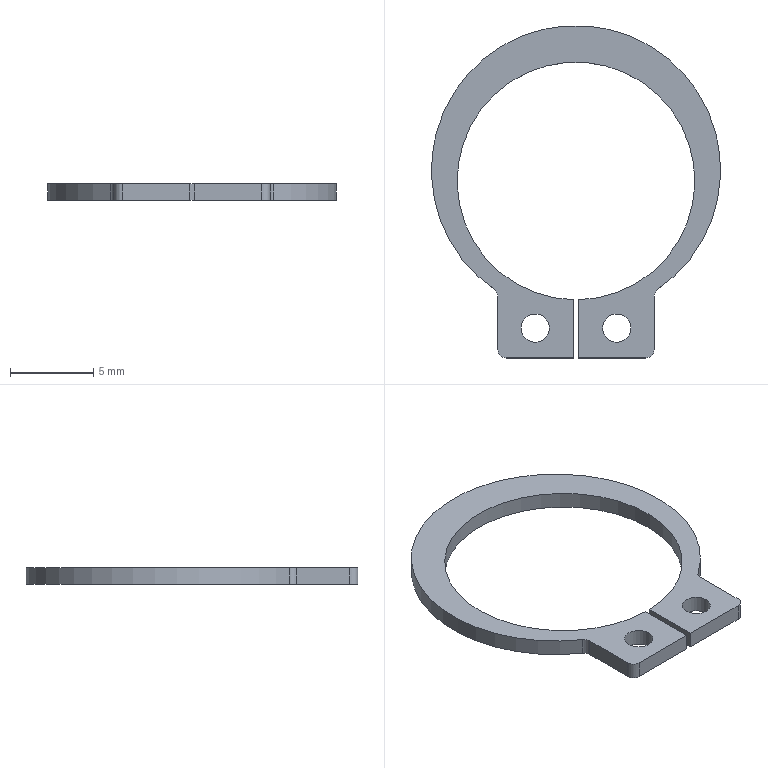Part | NX | features 5003_348_STWN15(Default) 2 | 1 solid | 16 faces | box 17.4 x 20 x 1 mm | volume 100.119 mm3 | cylinder 8 | plane 8 | commonest cylinder face diameters 1 x4 1.7 x2 14.3 x1 17.4 x1
STEP:
#1=CARTESIAN_POINT('',(163.225,-328.939,-258.15));
#2=VERTEX_POINT('',#1);
#3=CARTESIAN_POINT('',(163.442,-328.527,-258.15));
#4=VERTEX_POINT('',#3);
#5=CARTESIAN_POINT('',(163.725,-328.939,-258.15));
#6=DIRECTION('',(0.,0.,-1.));
#7=DIRECTION('',(-1.,0.,0.));
#8=AXIS2_PLACEMENT_3D('',#5,#6,#7);
#9=CIRCLE('',#8,0.5);
#10=EDGE_CURVE('',#2,#4,#9,.T.);
#11=ORIENTED_EDGE('',*,*,#10,.T.);
#12=CARTESIAN_POINT('',(163.442,-328.527,-257.15));
#13=VERTEX_POINT('',#12);
#14=CARTESIAN_POINT('',(163.442,-328.527,-257.15));
#15=DIRECTION('',(0.,0.,-1.));
#16=VECTOR('',#15,1000.);
#17=LINE('',#14,#16);
#18=EDGE_CURVE('',#13,#4,#17,.T.);
#19=ORIENTED_EDGE('',*,*,#18,.F.);
#20=CARTESIAN_POINT('',(163.225,-328.939,-257.15));
#21=VERTEX_POINT('',#20);
#22=CARTESIAN_POINT('',(163.725,-328.939,-257.15));
#23=DIRECTION('',(0.,0.,-1.));
#24=DIRECTION('',(-1.,0.,0.));
#25=AXIS2_PLACEMENT_3D('',#22,#23,#24);
#26=CIRCLE('',#25,0.5);
#27=EDGE_CURVE('',#21,#13,#26,.T.);
#28=ORIENTED_EDGE('',*,*,#27,.F.);
#29=CARTESIAN_POINT('',(163.225,-328.939,-257.15));
#30=DIRECTION('',(0.,0.,-1.));
#31=VECTOR('',#30,1000.);
#32=LINE('',#29,#31);
#33=EDGE_CURVE('',#21,#2,#32,.T.);
#34=ORIENTED_EDGE('',*,*,#33,.T.);
#35=EDGE_LOOP('',(#11,#19,#28,#34));
#36=FACE_BOUND('',#35,.T.);
#37=CARTESIAN_POINT('',(163.725,-328.939,-257.15));
#38=DIRECTION('',(0.,0.,-1.));
#39=DIRECTION('',(-1.,0.,0.));
#40=AXIS2_PLACEMENT_3D('',#37,#38,#39);
#41=CYLINDRICAL_SURFACE('',#40,0.5);
#42=ADVANCED_FACE('',(#36),#41,.F.);
#43=CARTESIAN_POINT('',(153.608,-328.527,-258.15));
#44=VERTEX_POINT('',#43);
#45=CARTESIAN_POINT('',(158.525,-321.35,-258.15));
#46=DIRECTION('',(0.,0.,1.));
#47=DIRECTION('',(1.,0.,0.));
#48=AXIS2_PLACEMENT_3D('',#45,#46,#47);
#49=CIRCLE('',#48,8.7);
#50=EDGE_CURVE('',#4,#44,#49,.T.);
#51=ORIENTED_EDGE('',*,*,#50,.T.);
#52=CARTESIAN_POINT('',(153.608,-328.527,-257.15));
#53=VERTEX_POINT('',#52);
#54=CARTESIAN_POINT('',(153.608,-328.527,-257.15));
#55=DIRECTION('',(0.,0.,-1.));
#56=VECTOR('',#55,1000.);
#57=LINE('',#54,#56);
#58=EDGE_CURVE('',#53,#44,#57,.T.);
#59=ORIENTED_EDGE('',*,*,#58,.F.);
#60=CARTESIAN_POINT('',(158.525,-321.35,-257.15));
#61=DIRECTION('',(0.,0.,1.));
#62=DIRECTION('',(1.,0.,0.));
#63=AXIS2_PLACEMENT_3D('',#60,#61,#62);
#64=CIRCLE('',#63,8.7);
#65=EDGE_CURVE('',#13,#53,#64,.T.);
#66=ORIENTED_EDGE('',*,*,#65,.F.);
#67=ORIENTED_EDGE('',*,*,#18,.T.);
#68=EDGE_LOOP('',(#51,#59,#66,#67));
#69=FACE_BOUND('',#68,.T.);
#70=CARTESIAN_POINT('',(158.525,-321.35,-257.15));
#71=DIRECTION('',(0.,0.,-1.));
#72=DIRECTION('',(-1.,0.,0.));
#73=AXIS2_PLACEMENT_3D('',#70,#71,#72);
#74=CYLINDRICAL_SURFACE('',#73,8.7);
#75=ADVANCED_FACE('',(#69),#74,.T.);
#76=CARTESIAN_POINT('',(153.825,-328.939,-258.15));
#77=VERTEX_POINT('',#76);
#78=CARTESIAN_POINT('',(153.325,-328.939,-258.15));
#79=DIRECTION('',(0.,0.,-1.));
#80=DIRECTION('',(-1.,0.,0.));
#81=AXIS2_PLACEMENT_3D('',#78,#79,#80);
#82=CIRCLE('',#81,0.5);
#83=EDGE_CURVE('',#44,#77,#82,.T.);
#84=ORIENTED_EDGE('',*,*,#83,.T.);
#85=CARTESIAN_POINT('',(153.825,-328.939,-257.15));
#86=VERTEX_POINT('',#85);
#87=CARTESIAN_POINT('',(153.825,-328.939,-257.15));
#88=DIRECTION('',(0.,0.,-1.));
#89=VECTOR('',#88,1000.);
#90=LINE('',#87,#89);
#91=EDGE_CURVE('',#86,#77,#90,.T.);
#92=ORIENTED_EDGE('',*,*,#91,.F.);
#93=CARTESIAN_POINT('',(153.325,-328.939,-257.15));
#94=DIRECTION('',(0.,0.,-1.));
#95=DIRECTION('',(-1.,0.,0.));
#96=AXIS2_PLACEMENT_3D('',#93,#94,#95);
#97=CIRCLE('',#96,0.5);
#98=EDGE_CURVE('',#53,#86,#97,.T.);
#99=ORIENTED_EDGE('',*,*,#98,.F.);
#100=ORIENTED_EDGE('',*,*,#58,.T.);
#101=EDGE_LOOP('',(#84,#92,#99,#100));
#102=FACE_BOUND('',#101,.T.);
#103=CARTESIAN_POINT('',(153.325,-328.939,-257.15));
#104=DIRECTION('',(0.,0.,-1.));
#105=DIRECTION('',(-1.,0.,0.));
#106=AXIS2_PLACEMENT_3D('',#103,#104,#105);
#107=CYLINDRICAL_SURFACE('',#106,0.5);
#108=ADVANCED_FACE('',(#102),#107,.F.);
#109=CARTESIAN_POINT('',(153.825,-332.15,-258.15));
#110=VERTEX_POINT('',#109);
#111=CARTESIAN_POINT('',(153.825,-328.939,-258.15));
#112=DIRECTION('',(0.,-1.,0.));
#113=VECTOR('',#112,1000.);
#114=LINE('',#111,#113);
#115=EDGE_CURVE('',#77,#110,#114,.T.);
#116=ORIENTED_EDGE('',*,*,#115,.T.);
#117=CARTESIAN_POINT('',(153.825,-332.15,-257.15));
#118=VERTEX_POINT('',#117);
#119=CARTESIAN_POINT('',(153.825,-332.15,-257.15));
#120=DIRECTION('',(0.,0.,-1.));
#121=VECTOR('',#120,1000.);
#122=LINE('',#119,#121);
#123=EDGE_CURVE('',#118,#110,#122,.T.);
#124=ORIENTED_EDGE('',*,*,#123,.F.);
#125=CARTESIAN_POINT('',(153.825,-328.939,-257.15));
#126=DIRECTION('',(0.,-1.,0.));
#127=VECTOR('',#126,1000.);
#128=LINE('',#125,#127);
#129=EDGE_CURVE('',#86,#118,#128,.T.);
#130=ORIENTED_EDGE('',*,*,#129,.F.);
#131=ORIENTED_EDGE('',*,*,#91,.T.);
#132=EDGE_LOOP('',(#116,#124,#130,#131));
#133=FACE_BOUND('',#132,.T.);
#134=CARTESIAN_POINT('',(153.825,-328.939,-257.15));
#135=DIRECTION('',(1.,0.,0.));
#136=DIRECTION('',(0.,1.,0.));
#137=AXIS2_PLACEMENT_3D('',#134,#135,#136);
#138=PLANE('',#137);
#139=ADVANCED_FACE('',(#133),#138,.F.);
#140=CARTESIAN_POINT('',(154.325,-332.65,-258.15));
#141=VERTEX_POINT('',#140);
#142=CARTESIAN_POINT('',(154.325,-332.15,-258.15));
#143=DIRECTION('',(0.,0.,1.));
#144=DIRECTION('',(1.,0.,0.));
#145=AXIS2_PLACEMENT_3D('',#142,#143,#144);
#146=CIRCLE('',#145,0.5);
#147=EDGE_CURVE('',#110,#141,#146,.T.);
#148=ORIENTED_EDGE('',*,*,#147,.T.);
#149=CARTESIAN_POINT('',(154.325,-332.65,-257.15));
#150=VERTEX_POINT('',#149);
#151=CARTESIAN_POINT('',(154.325,-332.65,-257.15));
#152=DIRECTION('',(0.,0.,-1.));
#153=VECTOR('',#152,1000.);
#154=LINE('',#151,#153);
#155=EDGE_CURVE('',#150,#141,#154,.T.);
#156=ORIENTED_EDGE('',*,*,#155,.F.);
#157=CARTESIAN_POINT('',(154.325,-332.15,-257.15));
#158=DIRECTION('',(0.,0.,1.));
#159=DIRECTION('',(1.,0.,0.));
#160=AXIS2_PLACEMENT_3D('',#157,#158,#159);
#161=CIRCLE('',#160,0.5);
#162=EDGE_CURVE('',#118,#150,#161,.T.);
#163=ORIENTED_EDGE('',*,*,#162,.F.);
#164=ORIENTED_EDGE('',*,*,#123,.T.);
#165=EDGE_LOOP('',(#148,#156,#163,#164));
#166=FACE_BOUND('',#165,.T.);
#167=CARTESIAN_POINT('',(154.325,-332.15,-257.15));
#168=DIRECTION('',(0.,0.,-1.));
#169=DIRECTION('',(-1.,0.,0.));
#170=AXIS2_PLACEMENT_3D('',#167,#168,#169);
#171=CYLINDRICAL_SURFACE('',#170,0.5);
#172=ADVANCED_FACE('',(#166),#171,.T.);
#173=CARTESIAN_POINT('',(158.375,-332.65,-258.15));
#174=VERTEX_POINT('',#173);
#175=CARTESIAN_POINT('',(154.325,-332.65,-258.15));
#176=DIRECTION('',(1.,0.,0.));
#177=VECTOR('',#176,1000.);
#178=LINE('',#175,#177);
#179=EDGE_CURVE('',#141,#174,#178,.T.);
#180=ORIENTED_EDGE('',*,*,#179,.T.);
#181=CARTESIAN_POINT('',(158.375,-332.65,-257.15));
#182=VERTEX_POINT('',#181);
#183=CARTESIAN_POINT('',(158.375,-332.65,-257.15));
#184=DIRECTION('',(0.,0.,-1.));
#185=VECTOR('',#184,1000.);
#186=LINE('',#183,#185);
#187=EDGE_CURVE('',#182,#174,#186,.T.);
#188=ORIENTED_EDGE('',*,*,#187,.F.);
#189=CARTESIAN_POINT('',(154.325,-332.65,-257.15));
#190=DIRECTION('',(1.,0.,0.));
#191=VECTOR('',#190,1000.);
#192=LINE('',#189,#191);
#193=EDGE_CURVE('',#150,#182,#192,.T.);
#194=ORIENTED_EDGE('',*,*,#193,.F.);
#195=ORIENTED_EDGE('',*,*,#155,.T.);
#196=EDGE_LOOP('',(#180,#188,#194,#195));
#197=FACE_BOUND('',#196,.T.);
#198=CARTESIAN_POINT('',(154.325,-332.65,-257.15));
#199=DIRECTION('',(0.,1.,0.));
#200=DIRECTION('',(0.,0.,1.));
#201=AXIS2_PLACEMENT_3D('',#198,#199,#200);
#202=PLANE('',#201);
#203=ADVANCED_FACE('',(#197),#202,.F.);
#204=CARTESIAN_POINT('',(158.375,-329.148,-258.15));
#205=VERTEX_POINT('',#204);
#206=CARTESIAN_POINT('',(158.375,-332.65,-258.15));
#207=DIRECTION('',(0.,1.,0.));
#208=VECTOR('',#207,1000.);
#209=LINE('',#206,#208);
#210=EDGE_CURVE('',#174,#205,#209,.T.);
#211=ORIENTED_EDGE('',*,*,#210,.T.);
#212=CARTESIAN_POINT('',(158.375,-329.148,-257.15));
#213=VERTEX_POINT('',#212);
#214=CARTESIAN_POINT('',(158.375,-329.148,-257.15));
#215=DIRECTION('',(0.,0.,-1.));
#216=VECTOR('',#215,1000.);
#217=LINE('',#214,#216);
#218=EDGE_CURVE('',#213,#205,#217,.T.);
#219=ORIENTED_EDGE('',*,*,#218,.F.);
#220=CARTESIAN_POINT('',(158.375,-332.65,-257.15));
#221=DIRECTION('',(0.,1.,0.));
#222=VECTOR('',#221,1000.);
#223=LINE('',#220,#222);
#224=EDGE_CURVE('',#182,#213,#223,.T.);
#225=ORIENTED_EDGE('',*,*,#224,.F.);
#226=ORIENTED_EDGE('',*,*,#187,.T.);
#227=EDGE_LOOP('',(#211,#219,#225,#226));
#228=FACE_BOUND('',#227,.T.);
#229=CARTESIAN_POINT('',(158.375,-332.65,-257.15));
#230=DIRECTION('',(-1.,0.,0.));
#231=DIRECTION('',(0.,-1.,0.));
#232=AXIS2_PLACEMENT_3D('',#229,#230,#231);
#233=PLANE('',#232);
#234=ADVANCED_FACE('',(#228),#233,.F.);
#235=CARTESIAN_POINT('',(158.675,-329.148,-258.15));
#236=VERTEX_POINT('',#235);
#237=CARTESIAN_POINT('',(158.525,-322.,-258.15));
#238=DIRECTION('',(0.,0.,-1.));
#239=DIRECTION('',(-1.,0.,0.));
#240=AXIS2_PLACEMENT_3D('',#237,#238,#239);
#241=CIRCLE('',#240,7.15);
#242=EDGE_CURVE('',#205,#236,#241,.T.);
#243=ORIENTED_EDGE('',*,*,#242,.T.);
#244=CARTESIAN_POINT('',(158.675,-329.148,-257.15));
#245=VERTEX_POINT('',#244);
#246=CARTESIAN_POINT('',(158.675,-329.148,-257.15));
#247=DIRECTION('',(0.,0.,-1.));
#248=VECTOR('',#247,1000.);
#249=LINE('',#246,#248);
#250=EDGE_CURVE('',#245,#236,#249,.T.);
#251=ORIENTED_EDGE('',*,*,#250,.F.);
#252=CARTESIAN_POINT('',(158.525,-322.,-257.15));
#253=DIRECTION('',(0.,0.,-1.));
#254=DIRECTION('',(-1.,0.,0.));
#255=AXIS2_PLACEMENT_3D('',#252,#253,#254);
#256=CIRCLE('',#255,7.15);
#257=EDGE_CURVE('',#213,#245,#256,.T.);
#258=ORIENTED_EDGE('',*,*,#257,.F.);
#259=ORIENTED_EDGE('',*,*,#218,.T.);
#260=EDGE_LOOP('',(#243,#251,#258,#259));
#261=FACE_BOUND('',#260,.T.);
#262=CARTESIAN_POINT('',(158.525,-322.,-257.15));
#263=DIRECTION('',(0.,0.,-1.));
#264=DIRECTION('',(-1.,0.,0.));
#265=AXIS2_PLACEMENT_3D('',#262,#263,#264);
#266=CYLINDRICAL_SURFACE('',#265,7.15);
#267=ADVANCED_FACE('',(#261),#266,.F.);
#268=CARTESIAN_POINT('',(158.675,-332.65,-258.15));
#269=VERTEX_POINT('',#268);
#270=CARTESIAN_POINT('',(158.675,-329.148,-258.15));
#271=DIRECTION('',(0.,-1.,0.));
#272=VECTOR('',#271,1000.);
#273=LINE('',#270,#272);
#274=EDGE_CURVE('',#236,#269,#273,.T.);
#275=ORIENTED_EDGE('',*,*,#274,.T.);
#276=CARTESIAN_POINT('',(158.675,-332.65,-257.15));
#277=VERTEX_POINT('',#276);
#278=CARTESIAN_POINT('',(158.675,-332.65,-257.15));
#279=DIRECTION('',(0.,0.,-1.));
#280=VECTOR('',#279,1000.);
#281=LINE('',#278,#280);
#282=EDGE_CURVE('',#277,#269,#281,.T.);
#283=ORIENTED_EDGE('',*,*,#282,.F.);
#284=CARTESIAN_POINT('',(158.675,-329.148,-257.15));
#285=DIRECTION('',(0.,-1.,0.));
#286=VECTOR('',#285,1000.);
#287=LINE('',#284,#286);
#288=EDGE_CURVE('',#245,#277,#287,.T.);
#289=ORIENTED_EDGE('',*,*,#288,.F.);
#290=ORIENTED_EDGE('',*,*,#250,.T.);
#291=EDGE_LOOP('',(#275,#283,#289,#290));
#292=FACE_BOUND('',#291,.T.);
#293=CARTESIAN_POINT('',(158.675,-329.148,-257.15));
#294=DIRECTION('',(1.,0.,0.));
#295=DIRECTION('',(0.,1.,0.));
#296=AXIS2_PLACEMENT_3D('',#293,#294,#295);
#297=PLANE('',#296);
#298=ADVANCED_FACE('',(#292),#297,.F.);
#299=CARTESIAN_POINT('',(162.725,-332.65,-258.15));
#300=VERTEX_POINT('',#299);
#301=CARTESIAN_POINT('',(158.675,-332.65,-258.15));
#302=DIRECTION('',(1.,0.,0.));
#303=VECTOR('',#302,1000.);
#304=LINE('',#301,#303);
#305=EDGE_CURVE('',#269,#300,#304,.T.);
#306=ORIENTED_EDGE('',*,*,#305,.T.);
#307=CARTESIAN_POINT('',(162.725,-332.65,-257.15));
#308=VERTEX_POINT('',#307);
#309=CARTESIAN_POINT('',(162.725,-332.65,-257.15));
#310=DIRECTION('',(0.,0.,-1.));
#311=VECTOR('',#310,1000.);
#312=LINE('',#309,#311);
#313=EDGE_CURVE('',#308,#300,#312,.T.);
#314=ORIENTED_EDGE('',*,*,#313,.F.);
#315=CARTESIAN_POINT('',(158.675,-332.65,-257.15));
#316=DIRECTION('',(1.,0.,0.));
#317=VECTOR('',#316,1000.);
#318=LINE('',#315,#317);
#319=EDGE_CURVE('',#277,#308,#318,.T.);
#320=ORIENTED_EDGE('',*,*,#319,.F.);
#321=ORIENTED_EDGE('',*,*,#282,.T.);
#322=EDGE_LOOP('',(#306,#314,#320,#321));
#323=FACE_BOUND('',#322,.T.);
#324=CARTESIAN_POINT('',(158.675,-332.65,-257.15));
#325=DIRECTION('',(0.,1.,0.));
#326=DIRECTION('',(0.,0.,1.));
#327=AXIS2_PLACEMENT_3D('',#324,#325,#326);
#328=PLANE('',#327);
#329=ADVANCED_FACE('',(#323),#328,.F.);
#330=CARTESIAN_POINT('',(163.225,-332.15,-258.15));
#331=VERTEX_POINT('',#330);
#332=CARTESIAN_POINT('',(162.725,-332.15,-258.15));
#333=DIRECTION('',(0.,0.,1.));
#334=DIRECTION('',(1.,0.,0.));
#335=AXIS2_PLACEMENT_3D('',#332,#333,#334);
#336=CIRCLE('',#335,0.5);
#337=EDGE_CURVE('',#300,#331,#336,.T.);
#338=ORIENTED_EDGE('',*,*,#337,.T.);
#339=CARTESIAN_POINT('',(163.225,-332.15,-257.15));
#340=VERTEX_POINT('',#339);
#341=CARTESIAN_POINT('',(163.225,-332.15,-257.15));
#342=DIRECTION('',(0.,0.,-1.));
#343=VECTOR('',#342,1000.);
#344=LINE('',#341,#343);
#345=EDGE_CURVE('',#340,#331,#344,.T.);
#346=ORIENTED_EDGE('',*,*,#345,.F.);
#347=CARTESIAN_POINT('',(162.725,-332.15,-257.15));
#348=DIRECTION('',(0.,0.,1.));
#349=DIRECTION('',(1.,0.,0.));
#350=AXIS2_PLACEMENT_3D('',#347,#348,#349);
#351=CIRCLE('',#350,0.5);
#352=EDGE_CURVE('',#308,#340,#351,.T.);
#353=ORIENTED_EDGE('',*,*,#352,.F.);
#354=ORIENTED_EDGE('',*,*,#313,.T.);
#355=EDGE_LOOP('',(#338,#346,#353,#354));
#356=FACE_BOUND('',#355,.T.);
#357=CARTESIAN_POINT('',(162.725,-332.15,-257.15));
#358=DIRECTION('',(0.,0.,-1.));
#359=DIRECTION('',(-1.,0.,0.));
#360=AXIS2_PLACEMENT_3D('',#357,#358,#359);
#361=CYLINDRICAL_SURFACE('',#360,0.5);
#362=ADVANCED_FACE('',(#356),#361,.T.);
#363=CARTESIAN_POINT('',(163.225,-332.15,-258.15));
#364=DIRECTION('',(0.,1.,0.));
#365=VECTOR('',#364,1000.);
#366=LINE('',#363,#365);
#367=EDGE_CURVE('',#331,#2,#366,.T.);
#368=ORIENTED_EDGE('',*,*,#367,.T.);
#369=ORIENTED_EDGE('',*,*,#33,.F.);
#370=CARTESIAN_POINT('',(163.225,-332.15,-257.15));
#371=DIRECTION('',(0.,1.,0.));
#372=VECTOR('',#371,1000.);
#373=LINE('',#370,#372);
#374=EDGE_CURVE('',#340,#21,#373,.T.);
#375=ORIENTED_EDGE('',*,*,#374,.F.);
#376=ORIENTED_EDGE('',*,*,#345,.T.);
#377=EDGE_LOOP('',(#368,#369,#375,#376));
#378=FACE_BOUND('',#377,.T.);
#379=CARTESIAN_POINT('',(163.225,-332.15,-257.15));
#380=DIRECTION('',(-1.,0.,0.));
#381=DIRECTION('',(0.,-1.,0.));
#382=AXIS2_PLACEMENT_3D('',#379,#380,#381);
#383=PLANE('',#382);
#384=ADVANCED_FACE('',(#378),#383,.F.);
#385=CARTESIAN_POINT('',(155.225,-330.85,-257.15));
#386=VERTEX_POINT('',#385);
#387=CARTESIAN_POINT('',(156.075,-330.85,-257.15));
#388=DIRECTION('',(0.,0.,-1.));
#389=DIRECTION('',(-1.,0.,0.));
#390=AXIS2_PLACEMENT_3D('',#387,#388,#389);
#391=CIRCLE('',#390,0.85);
#392=EDGE_CURVE('',#386,#386,#391,.T.);
#393=ORIENTED_EDGE('',*,*,#392,.T.);
#394=EDGE_LOOP('',(#393));
#395=FACE_BOUND('',#394,.T.);
#396=CARTESIAN_POINT('',(160.125,-330.85,-257.15));
#397=VERTEX_POINT('',#396);
#398=CARTESIAN_POINT('',(160.975,-330.85,-257.15));
#399=DIRECTION('',(0.,0.,-1.));
#400=DIRECTION('',(-1.,0.,0.));
#401=AXIS2_PLACEMENT_3D('',#398,#399,#400);
#402=CIRCLE('',#401,0.85);
#403=EDGE_CURVE('',#397,#397,#402,.T.);
#404=ORIENTED_EDGE('',*,*,#403,.T.);
#405=EDGE_LOOP('',(#404));
#406=FACE_BOUND('',#405,.T.);
#407=ORIENTED_EDGE('',*,*,#27,.T.);
#408=ORIENTED_EDGE('',*,*,#65,.T.);
#409=ORIENTED_EDGE('',*,*,#98,.T.);
#410=ORIENTED_EDGE('',*,*,#129,.T.);
#411=ORIENTED_EDGE('',*,*,#162,.T.);
#412=ORIENTED_EDGE('',*,*,#193,.T.);
#413=ORIENTED_EDGE('',*,*,#224,.T.);
#414=ORIENTED_EDGE('',*,*,#257,.T.);
#415=ORIENTED_EDGE('',*,*,#288,.T.);
#416=ORIENTED_EDGE('',*,*,#319,.T.);
#417=ORIENTED_EDGE('',*,*,#352,.T.);
#418=ORIENTED_EDGE('',*,*,#374,.T.);
#419=EDGE_LOOP('',(#407,#408,#409,#410,#411,#412,#413,#414,#415,#416,#417,#418));
#420=FACE_BOUND('',#419,.T.);
#421=CARTESIAN_POINT('',(163.725,-328.939,-257.15));
#422=DIRECTION('',(0.,0.,-1.));
#423=DIRECTION('',(-1.,0.,0.));
#424=AXIS2_PLACEMENT_3D('',#421,#422,#423);
#425=PLANE('',#424);
#426=ADVANCED_FACE('',(#395,#406,#420),#425,.F.);
#427=CARTESIAN_POINT('',(155.225,-330.85,-258.15));
#428=VERTEX_POINT('',#427);
#429=CARTESIAN_POINT('',(156.075,-330.85,-258.15));
#430=DIRECTION('',(0.,0.,-1.));
#431=DIRECTION('',(-1.,0.,0.));
#432=AXIS2_PLACEMENT_3D('',#429,#430,#431);
#433=CIRCLE('',#432,0.85);
#434=EDGE_CURVE('',#428,#428,#433,.T.);
#435=ORIENTED_EDGE('',*,*,#434,.F.);
#436=EDGE_LOOP('',(#435));
#437=FACE_BOUND('',#436,.T.);
#438=CARTESIAN_POINT('',(160.125,-330.85,-258.15));
#439=VERTEX_POINT('',#438);
#440=CARTESIAN_POINT('',(160.975,-330.85,-258.15));
#441=DIRECTION('',(0.,0.,-1.));
#442=DIRECTION('',(-1.,0.,0.));
#443=AXIS2_PLACEMENT_3D('',#440,#441,#442);
#444=CIRCLE('',#443,0.85);
#445=EDGE_CURVE('',#439,#439,#444,.T.);
#446=ORIENTED_EDGE('',*,*,#445,.F.);
#447=EDGE_LOOP('',(#446));
#448=FACE_BOUND('',#447,.T.);
#449=ORIENTED_EDGE('',*,*,#10,.F.);
#450=ORIENTED_EDGE('',*,*,#367,.F.);
#451=ORIENTED_EDGE('',*,*,#337,.F.);
#452=ORIENTED_EDGE('',*,*,#305,.F.);
#453=ORIENTED_EDGE('',*,*,#274,.F.);
#454=ORIENTED_EDGE('',*,*,#242,.F.);
#455=ORIENTED_EDGE('',*,*,#210,.F.);
#456=ORIENTED_EDGE('',*,*,#179,.F.);
#457=ORIENTED_EDGE('',*,*,#147,.F.);
#458=ORIENTED_EDGE('',*,*,#115,.F.);
#459=ORIENTED_EDGE('',*,*,#83,.F.);
#460=ORIENTED_EDGE('',*,*,#50,.F.);
#461=EDGE_LOOP('',(#449,#450,#451,#452,#453,#454,#455,#456,#457,#458,#459,#460));
#462=FACE_BOUND('',#461,.T.);
#463=CARTESIAN_POINT('',(163.725,-328.939,-258.15));
#464=DIRECTION('',(0.,0.,-1.));
#465=DIRECTION('',(-1.,0.,0.));
#466=AXIS2_PLACEMENT_3D('',#463,#464,#465);
#467=PLANE('',#466);
#468=ADVANCED_FACE('',(#437,#448,#462),#467,.T.);
#469=ORIENTED_EDGE('',*,*,#403,.F.);
#470=EDGE_LOOP('',(#469));
#471=FACE_BOUND('',#470,.T.);
#472=ORIENTED_EDGE('',*,*,#445,.T.);
#473=EDGE_LOOP('',(#472));
#474=FACE_BOUND('',#473,.T.);
#475=CARTESIAN_POINT('',(160.975,-330.85,-257.15));
#476=DIRECTION('',(0.,0.,-1.));
#477=DIRECTION('',(-1.,0.,0.));
#478=AXIS2_PLACEMENT_3D('',#475,#476,#477);
#479=CYLINDRICAL_SURFACE('',#478,0.85);
#480=ADVANCED_FACE('',(#471,#474),#479,.F.);
#481=ORIENTED_EDGE('',*,*,#392,.F.);
#482=EDGE_LOOP('',(#481));
#483=FACE_BOUND('',#482,.T.);
#484=ORIENTED_EDGE('',*,*,#434,.T.);
#485=EDGE_LOOP('',(#484));
#486=FACE_BOUND('',#485,.T.);
#487=CARTESIAN_POINT('',(156.075,-330.85,-257.15));
#488=DIRECTION('',(0.,0.,-1.));
#489=DIRECTION('',(-1.,0.,0.));
#490=AXIS2_PLACEMENT_3D('',#487,#488,#489);
#491=CYLINDRICAL_SURFACE('',#490,0.85);
#492=ADVANCED_FACE('',(#483,#486),#491,.F.);
#493=CLOSED_SHELL('',(#42,#75,#108,#139,#172,#203,#234,#267,#298,#329,#362,#384,#426,#468,#480,#492));
#494=MANIFOLD_SOLID_BREP('',#493);
#495=(LENGTH_UNIT()NAMED_UNIT(*)SI_UNIT(.MILLI.,.METRE.));
#496=UNCERTAINTY_MEASURE_WITH_UNIT(LENGTH_MEASURE(0.00001),#495,'','');
#497=(NAMED_UNIT(*)PLANE_ANGLE_UNIT()SI_UNIT($,.RADIAN.));
#498=(NAMED_UNIT(*)SI_UNIT($,.STERADIAN.)SOLID_ANGLE_UNIT());
#499=(GEOMETRIC_REPRESENTATION_CONTEXT(3)GLOBAL_UNCERTAINTY_ASSIGNED_CONTEXT((#496))GLOBAL_UNIT_ASSIGNED_CONTEXT((#495,#497,#498))REPRESENTATION_CONTEXT('',''));
#500=ADVANCED_BREP_SHAPE_REPRESENTATION('',(#494),#499);